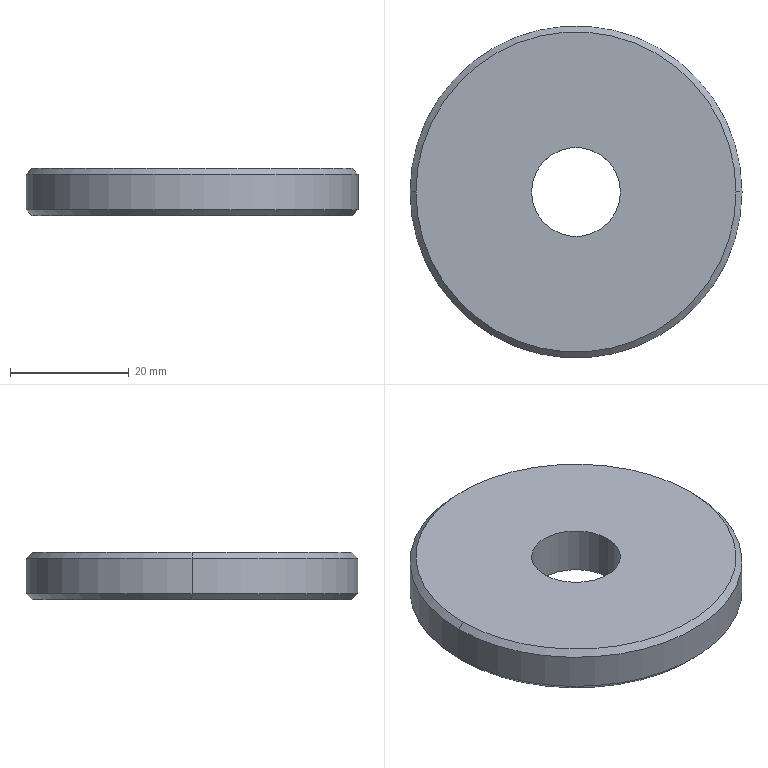Part | SolidWorks | features Chamfer 1, Extrusion 1 | 1 solid | 10 faces | box 56 x 56 x 8 mm | volume 18117 mm3 | cone 4 | cylinder 4 | plane 2 | commonest cylinder face diameters 15 x2 56 x2
STEP:
#1=CARTESIAN_POINT('',(27.,0.,8.));
#2=VERTEX_POINT('',#1);
#3=CARTESIAN_POINT('',(-27.,0.,8.));
#4=VERTEX_POINT('',#3);
#5=CARTESIAN_POINT('',(0.,0.,8.));
#6=DIRECTION('',(0.,0.,1.));
#7=DIRECTION('',(1.,0.,0.));
#8=AXIS2_PLACEMENT_3D('',#5,#6,#7);
#9=CIRCLE('',#8,27.);
#10=EDGE_CURVE('',#2,#4,#9,.T.);
#11=ORIENTED_EDGE('',*,*,#10,.F.);
#12=CARTESIAN_POINT('',(28.,0.,7.));
#13=VERTEX_POINT('',#12);
#14=CARTESIAN_POINT('',(27.,0.,8.));
#15=DIRECTION('',(0.7071,0.,-0.7071));
#16=VECTOR('',#15,1000.);
#17=LINE('',#14,#16);
#18=EDGE_CURVE('',#2,#13,#17,.T.);
#19=ORIENTED_EDGE('',*,*,#18,.T.);
#20=CARTESIAN_POINT('',(-28.,0.,7.));
#21=VERTEX_POINT('',#20);
#22=CARTESIAN_POINT('',(0.,0.,7.));
#23=DIRECTION('',(0.,0.,-1.));
#24=DIRECTION('',(1.,0.,0.));
#25=AXIS2_PLACEMENT_3D('',#22,#23,#24);
#26=CIRCLE('',#25,28.);
#27=EDGE_CURVE('',#21,#13,#26,.T.);
#28=ORIENTED_EDGE('',*,*,#27,.F.);
#29=CARTESIAN_POINT('',(-27.,0.,8.));
#30=DIRECTION('',(-0.7071,0.,-0.7071));
#31=VECTOR('',#30,1000.);
#32=LINE('',#29,#31);
#33=EDGE_CURVE('',#4,#21,#32,.T.);
#34=ORIENTED_EDGE('',*,*,#33,.F.);
#35=EDGE_LOOP('',(#11,#19,#28,#34));
#36=FACE_OUTER_BOUND('',#35,.T.);
#37=CARTESIAN_POINT('',(0.,0.,8.));
#38=DIRECTION('',(0.,0.,-1.));
#39=DIRECTION('',(-1.,0.,0.));
#40=AXIS2_PLACEMENT_3D('',#37,#38,#39);
#41=CONICAL_SURFACE('',#40,27.,0.7854);
#42=ADVANCED_FACE('',(#36),#41,.T.);
#43=CARTESIAN_POINT('',(-27.,0.,0.));
#44=VERTEX_POINT('',#43);
#45=CARTESIAN_POINT('',(27.,0.,0.));
#46=VERTEX_POINT('',#45);
#47=CARTESIAN_POINT('',(0.,0.,0.));
#48=DIRECTION('',(0.,0.,-1.));
#49=DIRECTION('',(1.,0.,0.));
#50=AXIS2_PLACEMENT_3D('',#47,#48,#49);
#51=CIRCLE('',#50,27.);
#52=EDGE_CURVE('',#44,#46,#51,.T.);
#53=ORIENTED_EDGE('',*,*,#52,.F.);
#54=CARTESIAN_POINT('',(-28.,0.,1.));
#55=VERTEX_POINT('',#54);
#56=CARTESIAN_POINT('',(-28.,0.,1.));
#57=DIRECTION('',(-0.7071,0.,0.7071));
#58=VECTOR('',#57,1000.);
#59=LINE('',#56,#58);
#60=EDGE_CURVE('',#44,#55,#59,.T.);
#61=ORIENTED_EDGE('',*,*,#60,.T.);
#62=CARTESIAN_POINT('',(28.,0.,1.));
#63=VERTEX_POINT('',#62);
#64=CARTESIAN_POINT('',(0.,0.,1.));
#65=DIRECTION('',(0.,0.,1.));
#66=DIRECTION('',(1.,0.,0.));
#67=AXIS2_PLACEMENT_3D('',#64,#65,#66);
#68=CIRCLE('',#67,28.);
#69=EDGE_CURVE('',#63,#55,#68,.T.);
#70=ORIENTED_EDGE('',*,*,#69,.F.);
#71=CARTESIAN_POINT('',(28.,0.,1.));
#72=DIRECTION('',(0.7071,0.,0.7071));
#73=VECTOR('',#72,1000.);
#74=LINE('',#71,#73);
#75=EDGE_CURVE('',#46,#63,#74,.T.);
#76=ORIENTED_EDGE('',*,*,#75,.F.);
#77=EDGE_LOOP('',(#53,#61,#70,#76));
#78=FACE_OUTER_BOUND('',#77,.T.);
#79=CARTESIAN_POINT('',(0.,0.,1.));
#80=DIRECTION('',(0.,0.,1.));
#81=DIRECTION('',(1.,0.,0.));
#82=AXIS2_PLACEMENT_3D('',#79,#80,#81);
#83=CONICAL_SURFACE('',#82,28.,0.7854);
#84=ADVANCED_FACE('',(#78),#83,.T.);
#85=CARTESIAN_POINT('',(-7.5,0.,8.));
#86=VERTEX_POINT('',#85);
#87=CARTESIAN_POINT('',(7.5,0.,8.));
#88=VERTEX_POINT('',#87);
#89=CARTESIAN_POINT('',(0.,0.,8.));
#90=DIRECTION('',(0.,0.,1.));
#91=DIRECTION('',(1.,0.,0.));
#92=AXIS2_PLACEMENT_3D('',#89,#90,#91);
#93=CIRCLE('',#92,7.5);
#94=EDGE_CURVE('',#86,#88,#93,.T.);
#95=ORIENTED_EDGE('',*,*,#94,.T.);
#96=CARTESIAN_POINT('',(7.5,0.,0.));
#97=VERTEX_POINT('',#96);
#98=CARTESIAN_POINT('',(7.5,0.,8.));
#99=DIRECTION('',(0.,0.,-1.));
#100=VECTOR('',#99,1000.);
#101=LINE('',#98,#100);
#102=EDGE_CURVE('',#88,#97,#101,.T.);
#103=ORIENTED_EDGE('',*,*,#102,.T.);
#104=CARTESIAN_POINT('',(-7.5,0.,0.));
#105=VERTEX_POINT('',#104);
#106=CARTESIAN_POINT('',(0.,0.,0.));
#107=DIRECTION('',(0.,0.,1.));
#108=DIRECTION('',(1.,0.,0.));
#109=AXIS2_PLACEMENT_3D('',#106,#107,#108);
#110=CIRCLE('',#109,7.5);
#111=EDGE_CURVE('',#105,#97,#110,.T.);
#112=ORIENTED_EDGE('',*,*,#111,.F.);
#113=CARTESIAN_POINT('',(-7.5,0.,8.));
#114=DIRECTION('',(0.,0.,-1.));
#115=VECTOR('',#114,1000.);
#116=LINE('',#113,#115);
#117=EDGE_CURVE('',#86,#105,#116,.T.);
#118=ORIENTED_EDGE('',*,*,#117,.F.);
#119=EDGE_LOOP('',(#95,#103,#112,#118));
#120=FACE_OUTER_BOUND('',#119,.T.);
#121=CARTESIAN_POINT('',(0.,0.,8.));
#122=DIRECTION('',(0.,0.,-1.));
#123=DIRECTION('',(-1.,0.,0.));
#124=AXIS2_PLACEMENT_3D('',#121,#122,#123);
#125=CYLINDRICAL_SURFACE('',#124,7.5);
#126=ADVANCED_FACE('',(#120),#125,.F.);
#127=ORIENTED_EDGE('',*,*,#27,.T.);
#128=CARTESIAN_POINT('',(28.,0.,8.));
#129=DIRECTION('',(0.,0.,-1.));
#130=VECTOR('',#129,1000.);
#131=LINE('',#128,#130);
#132=EDGE_CURVE('',#13,#63,#131,.T.);
#133=ORIENTED_EDGE('',*,*,#132,.T.);
#134=ORIENTED_EDGE('',*,*,#69,.T.);
#135=CARTESIAN_POINT('',(-28.,0.,8.));
#136=DIRECTION('',(0.,0.,-1.));
#137=VECTOR('',#136,1000.);
#138=LINE('',#135,#137);
#139=EDGE_CURVE('',#21,#55,#138,.T.);
#140=ORIENTED_EDGE('',*,*,#139,.F.);
#141=EDGE_LOOP('',(#127,#133,#134,#140));
#142=FACE_OUTER_BOUND('',#141,.T.);
#143=CARTESIAN_POINT('',(0.,0.,8.));
#144=DIRECTION('',(0.,0.,-1.));
#145=DIRECTION('',(-1.,0.,0.));
#146=AXIS2_PLACEMENT_3D('',#143,#144,#145);
#147=CYLINDRICAL_SURFACE('',#146,28.);
#148=ADVANCED_FACE('',(#142),#147,.T.);
#149=CARTESIAN_POINT('',(0.,0.,8.));
#150=DIRECTION('',(0.,0.,1.));
#151=DIRECTION('',(1.,0.,0.));
#152=AXIS2_PLACEMENT_3D('',#149,#150,#151);
#153=CIRCLE('',#152,27.);
#154=EDGE_CURVE('',#4,#2,#153,.T.);
#155=ORIENTED_EDGE('',*,*,#154,.T.);
#156=ORIENTED_EDGE('',*,*,#10,.T.);
#157=EDGE_LOOP('',(#155,#156));
#158=FACE_OUTER_BOUND('',#157,.T.);
#159=ORIENTED_EDGE('',*,*,#94,.F.);
#160=CARTESIAN_POINT('',(0.,0.,8.));
#161=DIRECTION('',(0.,0.,1.));
#162=DIRECTION('',(1.,0.,0.));
#163=AXIS2_PLACEMENT_3D('',#160,#161,#162);
#164=CIRCLE('',#163,7.5);
#165=EDGE_CURVE('',#88,#86,#164,.T.);
#166=ORIENTED_EDGE('',*,*,#165,.F.);
#167=EDGE_LOOP('',(#159,#166));
#168=FACE_BOUND('',#167,.T.);
#169=CARTESIAN_POINT('',(0.,0.,8.));
#170=DIRECTION('',(0.,0.,1.));
#171=DIRECTION('',(1.,0.,0.));
#172=AXIS2_PLACEMENT_3D('',#169,#170,#171);
#173=PLANE('',#172);
#174=ADVANCED_FACE('',(#158,#168),#173,.T.);
#175=CARTESIAN_POINT('',(0.,0.,0.));
#176=DIRECTION('',(0.,0.,-1.));
#177=DIRECTION('',(1.,0.,0.));
#178=AXIS2_PLACEMENT_3D('',#175,#176,#177);
#179=CIRCLE('',#178,27.);
#180=EDGE_CURVE('',#46,#44,#179,.T.);
#181=ORIENTED_EDGE('',*,*,#180,.T.);
#182=ORIENTED_EDGE('',*,*,#52,.T.);
#183=EDGE_LOOP('',(#181,#182));
#184=FACE_OUTER_BOUND('',#183,.T.);
#185=ORIENTED_EDGE('',*,*,#111,.T.);
#186=CARTESIAN_POINT('',(0.,0.,0.));
#187=DIRECTION('',(0.,0.,1.));
#188=DIRECTION('',(1.,0.,0.));
#189=AXIS2_PLACEMENT_3D('',#186,#187,#188);
#190=CIRCLE('',#189,7.5);
#191=EDGE_CURVE('',#97,#105,#190,.T.);
#192=ORIENTED_EDGE('',*,*,#191,.T.);
#193=EDGE_LOOP('',(#185,#192));
#194=FACE_BOUND('',#193,.T.);
#195=CARTESIAN_POINT('',(0.,0.,0.));
#196=DIRECTION('',(0.,0.,1.));
#197=DIRECTION('',(1.,0.,0.));
#198=AXIS2_PLACEMENT_3D('',#195,#196,#197);
#199=PLANE('',#198);
#200=ADVANCED_FACE('',(#184,#194),#199,.F.);
#201=ORIENTED_EDGE('',*,*,#132,.F.);
#202=CARTESIAN_POINT('',(0.,0.,7.));
#203=DIRECTION('',(0.,0.,-1.));
#204=DIRECTION('',(1.,0.,0.));
#205=AXIS2_PLACEMENT_3D('',#202,#203,#204);
#206=CIRCLE('',#205,28.);
#207=EDGE_CURVE('',#13,#21,#206,.T.);
#208=ORIENTED_EDGE('',*,*,#207,.T.);
#209=ORIENTED_EDGE('',*,*,#139,.T.);
#210=CARTESIAN_POINT('',(0.,0.,1.));
#211=DIRECTION('',(0.,0.,1.));
#212=DIRECTION('',(1.,0.,0.));
#213=AXIS2_PLACEMENT_3D('',#210,#211,#212);
#214=CIRCLE('',#213,28.);
#215=EDGE_CURVE('',#55,#63,#214,.T.);
#216=ORIENTED_EDGE('',*,*,#215,.T.);
#217=EDGE_LOOP('',(#201,#208,#209,#216));
#218=FACE_OUTER_BOUND('',#217,.T.);
#219=CARTESIAN_POINT('',(0.,0.,8.));
#220=DIRECTION('',(0.,0.,-1.));
#221=DIRECTION('',(-1.,0.,0.));
#222=AXIS2_PLACEMENT_3D('',#219,#220,#221);
#223=CYLINDRICAL_SURFACE('',#222,28.);
#224=ADVANCED_FACE('',(#218),#223,.T.);
#225=ORIENTED_EDGE('',*,*,#102,.F.);
#226=ORIENTED_EDGE('',*,*,#165,.T.);
#227=ORIENTED_EDGE('',*,*,#117,.T.);
#228=ORIENTED_EDGE('',*,*,#191,.F.);
#229=EDGE_LOOP('',(#225,#226,#227,#228));
#230=FACE_OUTER_BOUND('',#229,.T.);
#231=CARTESIAN_POINT('',(0.,0.,8.));
#232=DIRECTION('',(0.,0.,-1.));
#233=DIRECTION('',(-1.,0.,0.));
#234=AXIS2_PLACEMENT_3D('',#231,#232,#233);
#235=CYLINDRICAL_SURFACE('',#234,7.5);
#236=ADVANCED_FACE('',(#230),#235,.F.);
#237=ORIENTED_EDGE('',*,*,#60,.F.);
#238=ORIENTED_EDGE('',*,*,#180,.F.);
#239=ORIENTED_EDGE('',*,*,#75,.T.);
#240=ORIENTED_EDGE('',*,*,#215,.F.);
#241=EDGE_LOOP('',(#237,#238,#239,#240));
#242=FACE_OUTER_BOUND('',#241,.T.);
#243=CARTESIAN_POINT('',(0.,0.,1.));
#244=DIRECTION('',(0.,0.,1.));
#245=DIRECTION('',(1.,0.,0.));
#246=AXIS2_PLACEMENT_3D('',#243,#244,#245);
#247=CONICAL_SURFACE('',#246,28.,0.7854);
#248=ADVANCED_FACE('',(#242),#247,.T.);
#249=ORIENTED_EDGE('',*,*,#18,.F.);
#250=ORIENTED_EDGE('',*,*,#154,.F.);
#251=ORIENTED_EDGE('',*,*,#33,.T.);
#252=ORIENTED_EDGE('',*,*,#207,.F.);
#253=EDGE_LOOP('',(#249,#250,#251,#252));
#254=FACE_OUTER_BOUND('',#253,.T.);
#255=CARTESIAN_POINT('',(0.,0.,8.));
#256=DIRECTION('',(0.,0.,-1.));
#257=DIRECTION('',(-1.,0.,0.));
#258=AXIS2_PLACEMENT_3D('',#255,#256,#257);
#259=CONICAL_SURFACE('',#258,27.,0.7854);
#260=ADVANCED_FACE('',(#254),#259,.T.);
#261=CLOSED_SHELL('',(#42,#84,#126,#148,#174,#200,#224,#236,#248,#260));
#262=MANIFOLD_SOLID_BREP('',#261);
#263=CARTESIAN_POINT('',(0.,0.,0.));
#264=DIRECTION('',(0.,0.,1.));
#265=DIRECTION('',(1.,0.,0.));
#266=AXIS2_PLACEMENT_3D('',#263,#264,#265);
#267=(LENGTH_UNIT()NAMED_UNIT(*)SI_UNIT(.MILLI.,.METRE.));
#268=UNCERTAINTY_MEASURE_WITH_UNIT(LENGTH_MEASURE(0.00001),#267,'','');
#269=(NAMED_UNIT(*)PLANE_ANGLE_UNIT()SI_UNIT($,.RADIAN.));
#270=(NAMED_UNIT(*)SI_UNIT($,.STERADIAN.)SOLID_ANGLE_UNIT());
#271=(GEOMETRIC_REPRESENTATION_CONTEXT(3)GLOBAL_UNCERTAINTY_ASSIGNED_CONTEXT((#268))GLOBAL_UNIT_ASSIGNED_CONTEXT((#267,#269,#270))REPRESENTATION_CONTEXT('',''));
#272=ADVANCED_BREP_SHAPE_REPRESENTATION('',(#262,#266),#271);